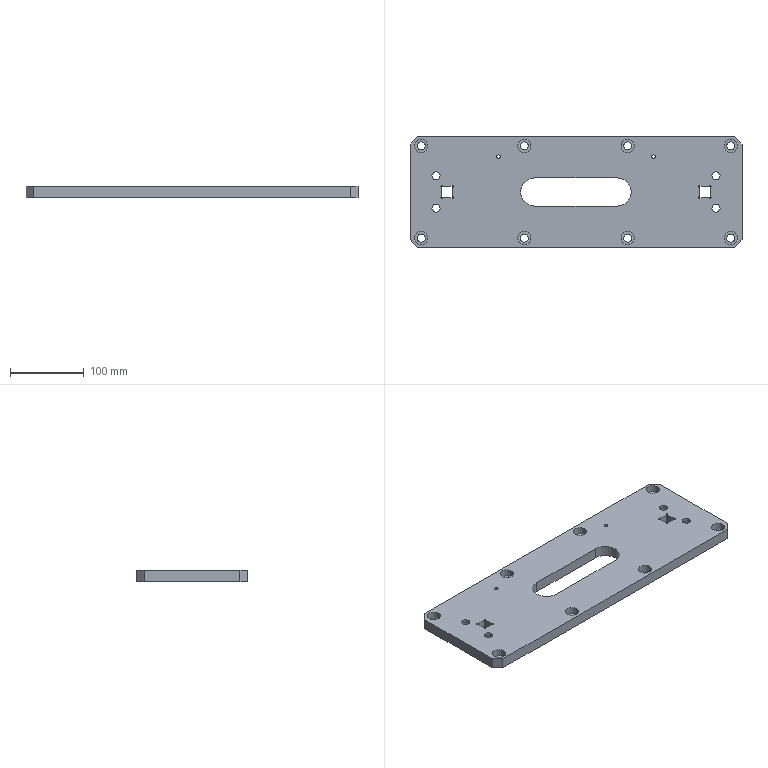Part | STEP file | Column base plate | 1 solid | 99 faces | box 450 x 150 x 15 mm | volume 884150 mm3 | cylinder 67 | plane 32 | commonest cylinder face diameters 11 x24 18 x24 2 x12 5 x4 38 x3